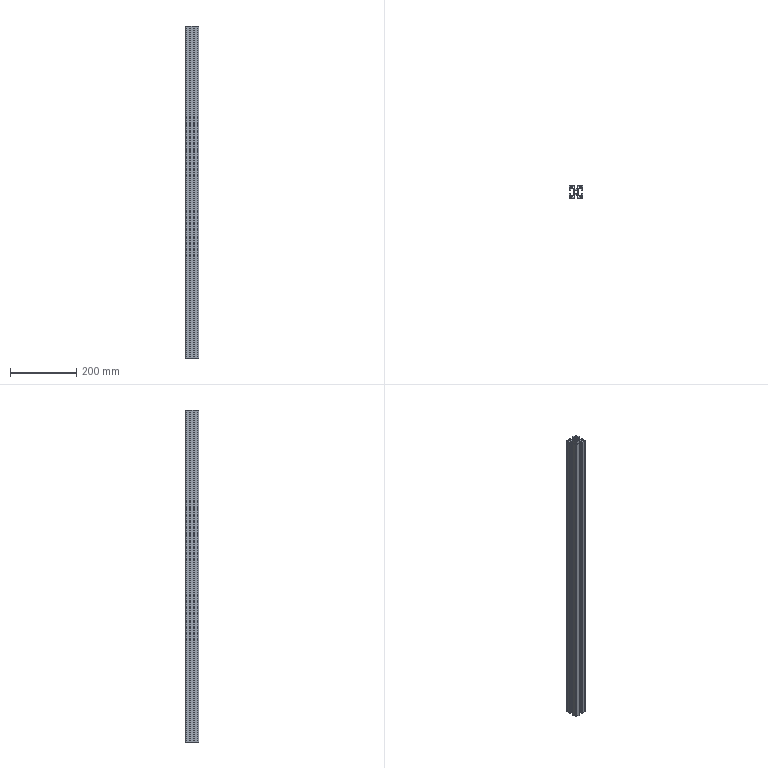Part | SolidWorks | features BaseBody 1 | 1 solid | 125 faces | box 40 x 40 x 1000 mm | volume 701466 mm3 | plane 74 | cylinder 51 | commonest cylinder face diameters 2 x24 1.5 x10 5 x8 10.2 x5 4 x4